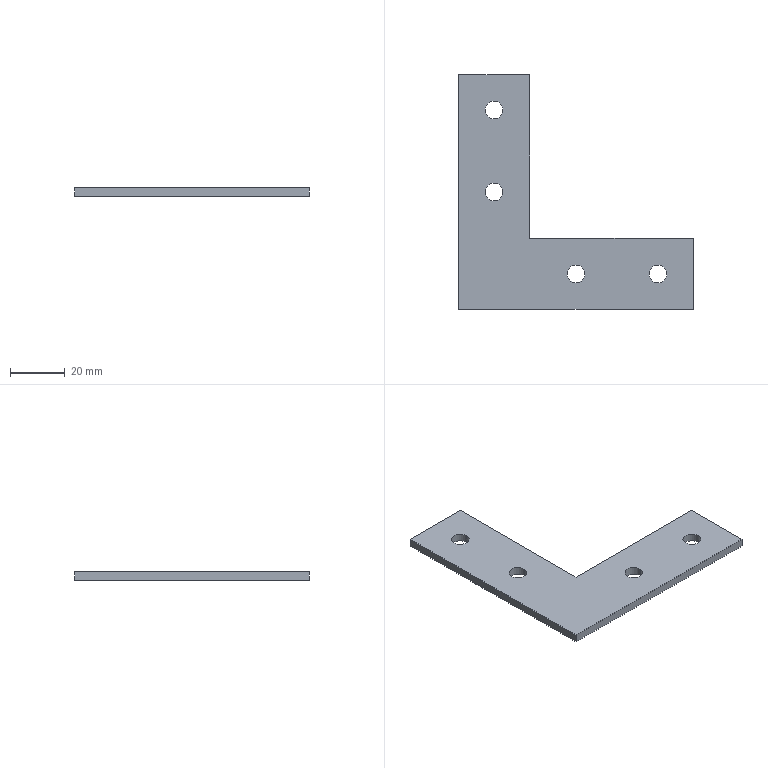Part | STEP file | Outer connecting plate | 1 solid | 16 faces | box 86 x 86 x 3 mm | volume 10990 mm3 | cylinder 8 | plane 8 | commonest cylinder face diameters 6.5 x8
STEP:
#1=CARTESIAN_POINT('',(0.,0.,0.));
#2=DIRECTION('',(0.,0.,1.));
#3=DIRECTION('',(1.,0.,0.));
#4=AXIS2_PLACEMENT_3D('',#1,#2,#3);
#5=CARTESIAN_POINT('',(16.25,73.,0.));
#6=VERTEX_POINT('',#5);
#7=CARTESIAN_POINT('',(16.25,73.,3.));
#8=VERTEX_POINT('',#7);
#9=CARTESIAN_POINT('',(16.25,73.,3.));
#10=DIRECTION('',(0.,0.,1.));
#11=VECTOR('',#10,1.);
#12=LINE('',#9,#11);
#13=CARTESIAN_POINT('',(13.,73.,3.));
#14=DIRECTION('',(0.,0.,1.));
#15=DIRECTION('',(1.,0.,0.));
#16=AXIS2_PLACEMENT_3D('',#13,#14,#15);
#17=CYLINDRICAL_SURFACE('',#16,3.25);
#18=CARTESIAN_POINT('',(6.283,0.));
#19=DIRECTION('',(0.,1.));
#20=VECTOR('',#19,1.);
#21=LINE('',#18,#20);
#22=(GEOMETRIC_REPRESENTATION_CONTEXT(2)PARAMETRIC_REPRESENTATION_CONTEXT()REPRESENTATION_CONTEXT('',''));
#23=DEFINITIONAL_REPRESENTATION('',(#21),#22);
#24=PCURVE('',#17,#23);
#25=CARTESIAN_POINT('',(13.,73.,3.));
#26=DIRECTION('',(0.,0.,1.));
#27=DIRECTION('',(1.,0.,0.));
#28=AXIS2_PLACEMENT_3D('',#25,#26,#27);
#29=CYLINDRICAL_SURFACE('',#28,3.25);
#30=CARTESIAN_POINT('',(0.,0.));
#31=DIRECTION('',(0.,1.));
#32=VECTOR('',#31,1.);
#33=LINE('',#30,#32);
#34=(GEOMETRIC_REPRESENTATION_CONTEXT(2)PARAMETRIC_REPRESENTATION_CONTEXT()REPRESENTATION_CONTEXT('',''));
#35=DEFINITIONAL_REPRESENTATION('',(#33),#34);
#36=PCURVE('',#29,#35);
#37=SURFACE_CURVE('',#12,(#24,#36),.PCURVE_S1.);
#38=EDGE_CURVE('',#6,#8,#37,.T.);
#39=ORIENTED_EDGE('',*,*,#38,.T.);
#40=CARTESIAN_POINT('',(9.75,73.,3.));
#41=VERTEX_POINT('',#40);
#42=CARTESIAN_POINT('',(13.,73.,3.));
#43=DIRECTION('',(0.,0.,1.));
#44=DIRECTION('',(1.,0.,0.));
#45=AXIS2_PLACEMENT_3D('',#42,#43,#44);
#46=CIRCLE('',#45,3.25);
#47=CARTESIAN_POINT('',(0.,0.));
#48=DIRECTION('',(1.,0.));
#49=VECTOR('',#48,1.);
#50=LINE('',#47,#49);
#51=(GEOMETRIC_REPRESENTATION_CONTEXT(2)PARAMETRIC_REPRESENTATION_CONTEXT()REPRESENTATION_CONTEXT('',''));
#52=DEFINITIONAL_REPRESENTATION('',(#50),#51);
#53=PCURVE('',#17,#52);
#54=CARTESIAN_POINT('',(0.,0.,3.));
#55=DIRECTION('',(0.,0.,-1.));
#56=DIRECTION('',(-1.,0.,0.));
#57=AXIS2_PLACEMENT_3D('',#54,#55,#56);
#58=PLANE('',#57);
#59=CARTESIAN_POINT('',(-16.25,73.));
#60=CARTESIAN_POINT('',(-16.25,78.629));
#61=CARTESIAN_POINT('',(-11.375,75.815));
#62=CARTESIAN_POINT('',(-6.5,73.));
#63=CARTESIAN_POINT('',(-11.375,70.185));
#64=CARTESIAN_POINT('',(-16.25,67.371));
#65=CARTESIAN_POINT('',(-16.25,73.));
#66=(BOUNDED_CURVE()B_SPLINE_CURVE(2,(#59,#60,#61,#62,#63,#64,#65),.UNSPECIFIED.,.T.,.F.)B_SPLINE_CURVE_WITH_KNOTS((1,2,2,2,2,1),(-2.094,0.,2.094,4.189,6.283,8.378),.UNSPECIFIED.)CURVE()GEOMETRIC_REPRESENTATION_ITEM()RATIONAL_B_SPLINE_CURVE((1.,0.5,1.,0.5,1.,0.5,1.))REPRESENTATION_ITEM(''));
#67=(GEOMETRIC_REPRESENTATION_CONTEXT(2)PARAMETRIC_REPRESENTATION_CONTEXT()REPRESENTATION_CONTEXT('',''));
#68=DEFINITIONAL_REPRESENTATION('',(#66),#67);
#69=PCURVE('',#58,#68);
#70=SURFACE_CURVE('',#46,(#53,#69),.PCURVE_S1.);
#71=EDGE_CURVE('',#41,#8,#70,.T.);
#72=ORIENTED_EDGE('',*,*,#71,.F.);
#73=CARTESIAN_POINT('',(9.75,73.,0.));
#74=VERTEX_POINT('',#73);
#75=CARTESIAN_POINT('',(9.75,73.,3.));
#76=DIRECTION('',(0.,0.,1.));
#77=VECTOR('',#76,1.);
#78=LINE('',#75,#77);
#79=CARTESIAN_POINT('',(3.142,0.));
#80=DIRECTION('',(0.,1.));
#81=VECTOR('',#80,1.);
#82=LINE('',#79,#81);
#83=(GEOMETRIC_REPRESENTATION_CONTEXT(2)PARAMETRIC_REPRESENTATION_CONTEXT()REPRESENTATION_CONTEXT('',''));
#84=DEFINITIONAL_REPRESENTATION('',(#82),#83);
#85=PCURVE('',#17,#84);
#86=CARTESIAN_POINT('',(3.142,0.));
#87=DIRECTION('',(0.,1.));
#88=VECTOR('',#87,1.);
#89=LINE('',#86,#88);
#90=(GEOMETRIC_REPRESENTATION_CONTEXT(2)PARAMETRIC_REPRESENTATION_CONTEXT()REPRESENTATION_CONTEXT('',''));
#91=DEFINITIONAL_REPRESENTATION('',(#89),#90);
#92=PCURVE('',#29,#91);
#93=SURFACE_CURVE('',#78,(#85,#92),.PCURVE_S1.);
#94=EDGE_CURVE('',#74,#41,#93,.T.);
#95=ORIENTED_EDGE('',*,*,#94,.F.);
#96=CARTESIAN_POINT('',(13.,73.,0.));
#97=DIRECTION('',(0.,0.,-1.));
#98=DIRECTION('',(-1.,0.,0.));
#99=AXIS2_PLACEMENT_3D('',#96,#97,#98);
#100=CIRCLE('',#99,3.25);
#101=CARTESIAN_POINT('',(9.425,-3.));
#102=DIRECTION('',(-1.,0.));
#103=VECTOR('',#102,1.);
#104=LINE('',#101,#103);
#105=(GEOMETRIC_REPRESENTATION_CONTEXT(2)PARAMETRIC_REPRESENTATION_CONTEXT()REPRESENTATION_CONTEXT('',''));
#106=DEFINITIONAL_REPRESENTATION('',(#104),#105);
#107=PCURVE('',#17,#106);
#108=CARTESIAN_POINT('',(0.,0.,0.));
#109=DIRECTION('',(0.,0.,-1.));
#110=DIRECTION('',(-1.,0.,0.));
#111=AXIS2_PLACEMENT_3D('',#108,#109,#110);
#112=PLANE('',#111);
#113=CARTESIAN_POINT('',(-13.,73.));
#114=DIRECTION('',(1.,0.));
#115=AXIS2_PLACEMENT_2D('',#113,#114);
#116=CIRCLE('',#115,3.25);
#117=(GEOMETRIC_REPRESENTATION_CONTEXT(2)PARAMETRIC_REPRESENTATION_CONTEXT()REPRESENTATION_CONTEXT('',''));
#118=DEFINITIONAL_REPRESENTATION('',(#116),#117);
#119=PCURVE('',#112,#118);
#120=SURFACE_CURVE('',#100,(#107,#119),.PCURVE_S1.);
#121=EDGE_CURVE('',#6,#74,#120,.T.);
#122=ORIENTED_EDGE('',*,*,#121,.F.);
#123=EDGE_LOOP('',(#39,#72,#95,#122));
#124=FACE_BOUND('',#123,.F.);
#125=ADVANCED_FACE('',(#124),#17,.F.);
#126=CARTESIAN_POINT('',(16.25,43.,0.));
#127=VERTEX_POINT('',#126);
#128=CARTESIAN_POINT('',(16.25,43.,3.));
#129=VERTEX_POINT('',#128);
#130=CARTESIAN_POINT('',(16.25,43.,3.));
#131=DIRECTION('',(0.,0.,1.));
#132=VECTOR('',#131,1.);
#133=LINE('',#130,#132);
#134=CARTESIAN_POINT('',(13.,43.,3.));
#135=DIRECTION('',(0.,0.,1.));
#136=DIRECTION('',(1.,0.,0.));
#137=AXIS2_PLACEMENT_3D('',#134,#135,#136);
#138=CYLINDRICAL_SURFACE('',#137,3.25);
#139=CARTESIAN_POINT('',(6.283,0.));
#140=DIRECTION('',(0.,1.));
#141=VECTOR('',#140,1.);
#142=LINE('',#139,#141);
#143=(GEOMETRIC_REPRESENTATION_CONTEXT(2)PARAMETRIC_REPRESENTATION_CONTEXT()REPRESENTATION_CONTEXT('',''));
#144=DEFINITIONAL_REPRESENTATION('',(#142),#143);
#145=PCURVE('',#138,#144);
#146=CARTESIAN_POINT('',(13.,43.,3.));
#147=DIRECTION('',(0.,0.,1.));
#148=DIRECTION('',(1.,0.,0.));
#149=AXIS2_PLACEMENT_3D('',#146,#147,#148);
#150=CYLINDRICAL_SURFACE('',#149,3.25);
#151=CARTESIAN_POINT('',(0.,0.));
#152=DIRECTION('',(0.,1.));
#153=VECTOR('',#152,1.);
#154=LINE('',#151,#153);
#155=(GEOMETRIC_REPRESENTATION_CONTEXT(2)PARAMETRIC_REPRESENTATION_CONTEXT()REPRESENTATION_CONTEXT('',''));
#156=DEFINITIONAL_REPRESENTATION('',(#154),#155);
#157=PCURVE('',#150,#156);
#158=SURFACE_CURVE('',#133,(#145,#157),.PCURVE_S1.);
#159=EDGE_CURVE('',#127,#129,#158,.T.);
#160=ORIENTED_EDGE('',*,*,#159,.T.);
#161=CARTESIAN_POINT('',(9.75,43.,3.));
#162=VERTEX_POINT('',#161);
#163=CARTESIAN_POINT('',(13.,43.,3.));
#164=DIRECTION('',(0.,0.,1.));
#165=DIRECTION('',(1.,0.,0.));
#166=AXIS2_PLACEMENT_3D('',#163,#164,#165);
#167=CIRCLE('',#166,3.25);
#168=CARTESIAN_POINT('',(0.,0.));
#169=DIRECTION('',(1.,0.));
#170=VECTOR('',#169,1.);
#171=LINE('',#168,#170);
#172=(GEOMETRIC_REPRESENTATION_CONTEXT(2)PARAMETRIC_REPRESENTATION_CONTEXT()REPRESENTATION_CONTEXT('',''));
#173=DEFINITIONAL_REPRESENTATION('',(#171),#172);
#174=PCURVE('',#138,#173);
#175=CARTESIAN_POINT('',(-16.25,43.));
#176=CARTESIAN_POINT('',(-16.25,48.629));
#177=CARTESIAN_POINT('',(-11.375,45.815));
#178=CARTESIAN_POINT('',(-6.5,43.));
#179=CARTESIAN_POINT('',(-11.375,40.185));
#180=CARTESIAN_POINT('',(-16.25,37.371));
#181=CARTESIAN_POINT('',(-16.25,43.));
#182=(BOUNDED_CURVE()B_SPLINE_CURVE(2,(#175,#176,#177,#178,#179,#180,#181),.UNSPECIFIED.,.T.,.F.)B_SPLINE_CURVE_WITH_KNOTS((1,2,2,2,2,1),(-2.094,0.,2.094,4.189,6.283,8.378),.UNSPECIFIED.)CURVE()GEOMETRIC_REPRESENTATION_ITEM()RATIONAL_B_SPLINE_CURVE((1.,0.5,1.,0.5,1.,0.5,1.))REPRESENTATION_ITEM(''));
#183=(GEOMETRIC_REPRESENTATION_CONTEXT(2)PARAMETRIC_REPRESENTATION_CONTEXT()REPRESENTATION_CONTEXT('',''));
#184=DEFINITIONAL_REPRESENTATION('',(#182),#183);
#185=PCURVE('',#58,#184);
#186=SURFACE_CURVE('',#167,(#174,#185),.PCURVE_S1.);
#187=EDGE_CURVE('',#162,#129,#186,.T.);
#188=ORIENTED_EDGE('',*,*,#187,.F.);
#189=CARTESIAN_POINT('',(9.75,43.,0.));
#190=VERTEX_POINT('',#189);
#191=CARTESIAN_POINT('',(9.75,43.,3.));
#192=DIRECTION('',(0.,0.,1.));
#193=VECTOR('',#192,1.);
#194=LINE('',#191,#193);
#195=CARTESIAN_POINT('',(3.142,0.));
#196=DIRECTION('',(0.,1.));
#197=VECTOR('',#196,1.);
#198=LINE('',#195,#197);
#199=(GEOMETRIC_REPRESENTATION_CONTEXT(2)PARAMETRIC_REPRESENTATION_CONTEXT()REPRESENTATION_CONTEXT('',''));
#200=DEFINITIONAL_REPRESENTATION('',(#198),#199);
#201=PCURVE('',#138,#200);
#202=CARTESIAN_POINT('',(3.142,0.));
#203=DIRECTION('',(0.,1.));
#204=VECTOR('',#203,1.);
#205=LINE('',#202,#204);
#206=(GEOMETRIC_REPRESENTATION_CONTEXT(2)PARAMETRIC_REPRESENTATION_CONTEXT()REPRESENTATION_CONTEXT('',''));
#207=DEFINITIONAL_REPRESENTATION('',(#205),#206);
#208=PCURVE('',#150,#207);
#209=SURFACE_CURVE('',#194,(#201,#208),.PCURVE_S1.);
#210=EDGE_CURVE('',#190,#162,#209,.T.);
#211=ORIENTED_EDGE('',*,*,#210,.F.);
#212=CARTESIAN_POINT('',(13.,43.,0.));
#213=DIRECTION('',(0.,0.,-1.));
#214=DIRECTION('',(-1.,0.,0.));
#215=AXIS2_PLACEMENT_3D('',#212,#213,#214);
#216=CIRCLE('',#215,3.25);
#217=CARTESIAN_POINT('',(9.425,-3.));
#218=DIRECTION('',(-1.,0.));
#219=VECTOR('',#218,1.);
#220=LINE('',#217,#219);
#221=(GEOMETRIC_REPRESENTATION_CONTEXT(2)PARAMETRIC_REPRESENTATION_CONTEXT()REPRESENTATION_CONTEXT('',''));
#222=DEFINITIONAL_REPRESENTATION('',(#220),#221);
#223=PCURVE('',#138,#222);
#224=CARTESIAN_POINT('',(-13.,43.));
#225=DIRECTION('',(1.,0.));
#226=AXIS2_PLACEMENT_2D('',#224,#225);
#227=CIRCLE('',#226,3.25);
#228=(GEOMETRIC_REPRESENTATION_CONTEXT(2)PARAMETRIC_REPRESENTATION_CONTEXT()REPRESENTATION_CONTEXT('',''));
#229=DEFINITIONAL_REPRESENTATION('',(#227),#228);
#230=PCURVE('',#112,#229);
#231=SURFACE_CURVE('',#216,(#223,#230),.PCURVE_S1.);
#232=EDGE_CURVE('',#127,#190,#231,.T.);
#233=ORIENTED_EDGE('',*,*,#232,.F.);
#234=EDGE_LOOP('',(#160,#188,#211,#233));
#235=FACE_BOUND('',#234,.F.);
#236=ADVANCED_FACE('',(#235),#138,.F.);
#237=CARTESIAN_POINT('',(46.25,13.,0.));
#238=VERTEX_POINT('',#237);
#239=CARTESIAN_POINT('',(46.25,13.,3.));
#240=VERTEX_POINT('',#239);
#241=CARTESIAN_POINT('',(46.25,13.,3.));
#242=DIRECTION('',(0.,0.,1.));
#243=VECTOR('',#242,1.);
#244=LINE('',#241,#243);
#245=CARTESIAN_POINT('',(43.,13.,3.));
#246=DIRECTION('',(0.,0.,1.));
#247=DIRECTION('',(1.,0.,0.));
#248=AXIS2_PLACEMENT_3D('',#245,#246,#247);
#249=CYLINDRICAL_SURFACE('',#248,3.25);
#250=CARTESIAN_POINT('',(6.283,0.));
#251=DIRECTION('',(0.,1.));
#252=VECTOR('',#251,1.);
#253=LINE('',#250,#252);
#254=(GEOMETRIC_REPRESENTATION_CONTEXT(2)PARAMETRIC_REPRESENTATION_CONTEXT()REPRESENTATION_CONTEXT('',''));
#255=DEFINITIONAL_REPRESENTATION('',(#253),#254);
#256=PCURVE('',#249,#255);
#257=CARTESIAN_POINT('',(43.,13.,3.));
#258=DIRECTION('',(0.,0.,1.));
#259=DIRECTION('',(1.,0.,0.));
#260=AXIS2_PLACEMENT_3D('',#257,#258,#259);
#261=CYLINDRICAL_SURFACE('',#260,3.25);
#262=CARTESIAN_POINT('',(0.,0.));
#263=DIRECTION('',(0.,1.));
#264=VECTOR('',#263,1.);
#265=LINE('',#262,#264);
#266=(GEOMETRIC_REPRESENTATION_CONTEXT(2)PARAMETRIC_REPRESENTATION_CONTEXT()REPRESENTATION_CONTEXT('',''));
#267=DEFINITIONAL_REPRESENTATION('',(#265),#266);
#268=PCURVE('',#261,#267);
#269=SURFACE_CURVE('',#244,(#256,#268),.PCURVE_S1.);
#270=EDGE_CURVE('',#238,#240,#269,.T.);
#271=ORIENTED_EDGE('',*,*,#270,.T.);
#272=CARTESIAN_POINT('',(39.75,13.,3.));
#273=VERTEX_POINT('',#272);
#274=CARTESIAN_POINT('',(43.,13.,3.));
#275=DIRECTION('',(0.,0.,1.));
#276=DIRECTION('',(1.,0.,0.));
#277=AXIS2_PLACEMENT_3D('',#274,#275,#276);
#278=CIRCLE('',#277,3.25);
#279=CARTESIAN_POINT('',(0.,0.));
#280=DIRECTION('',(1.,0.));
#281=VECTOR('',#280,1.);
#282=LINE('',#279,#281);
#283=(GEOMETRIC_REPRESENTATION_CONTEXT(2)PARAMETRIC_REPRESENTATION_CONTEXT()REPRESENTATION_CONTEXT('',''));
#284=DEFINITIONAL_REPRESENTATION('',(#282),#283);
#285=PCURVE('',#249,#284);
#286=CARTESIAN_POINT('',(-46.25,13.));
#287=CARTESIAN_POINT('',(-46.25,18.629));
#288=CARTESIAN_POINT('',(-41.375,15.815));
#289=CARTESIAN_POINT('',(-36.5,13.));
#290=CARTESIAN_POINT('',(-41.375,10.185));
#291=CARTESIAN_POINT('',(-46.25,7.371));
#292=CARTESIAN_POINT('',(-46.25,13.));
#293=(BOUNDED_CURVE()B_SPLINE_CURVE(2,(#286,#287,#288,#289,#290,#291,#292),.UNSPECIFIED.,.T.,.F.)B_SPLINE_CURVE_WITH_KNOTS((1,2,2,2,2,1),(-2.094,0.,2.094,4.189,6.283,8.378),.UNSPECIFIED.)CURVE()GEOMETRIC_REPRESENTATION_ITEM()RATIONAL_B_SPLINE_CURVE((1.,0.5,1.,0.5,1.,0.5,1.))REPRESENTATION_ITEM(''));
#294=(GEOMETRIC_REPRESENTATION_CONTEXT(2)PARAMETRIC_REPRESENTATION_CONTEXT()REPRESENTATION_CONTEXT('',''));
#295=DEFINITIONAL_REPRESENTATION('',(#293),#294);
#296=PCURVE('',#58,#295);
#297=SURFACE_CURVE('',#278,(#285,#296),.PCURVE_S1.);
#298=EDGE_CURVE('',#273,#240,#297,.T.);
#299=ORIENTED_EDGE('',*,*,#298,.F.);
#300=CARTESIAN_POINT('',(39.75,13.,0.));
#301=VERTEX_POINT('',#300);
#302=CARTESIAN_POINT('',(39.75,13.,3.));
#303=DIRECTION('',(0.,0.,1.));
#304=VECTOR('',#303,1.);
#305=LINE('',#302,#304);
#306=CARTESIAN_POINT('',(3.142,0.));
#307=DIRECTION('',(0.,1.));
#308=VECTOR('',#307,1.);
#309=LINE('',#306,#308);
#310=(GEOMETRIC_REPRESENTATION_CONTEXT(2)PARAMETRIC_REPRESENTATION_CONTEXT()REPRESENTATION_CONTEXT('',''));
#311=DEFINITIONAL_REPRESENTATION('',(#309),#310);
#312=PCURVE('',#249,#311);
#313=CARTESIAN_POINT('',(3.142,0.));
#314=DIRECTION('',(0.,1.));
#315=VECTOR('',#314,1.);
#316=LINE('',#313,#315);
#317=(GEOMETRIC_REPRESENTATION_CONTEXT(2)PARAMETRIC_REPRESENTATION_CONTEXT()REPRESENTATION_CONTEXT('',''));
#318=DEFINITIONAL_REPRESENTATION('',(#316),#317);
#319=PCURVE('',#261,#318);
#320=SURFACE_CURVE('',#305,(#312,#319),.PCURVE_S1.);
#321=EDGE_CURVE('',#301,#273,#320,.T.);
#322=ORIENTED_EDGE('',*,*,#321,.F.);
#323=CARTESIAN_POINT('',(43.,13.,0.));
#324=DIRECTION('',(0.,0.,-1.));
#325=DIRECTION('',(-1.,0.,0.));
#326=AXIS2_PLACEMENT_3D('',#323,#324,#325);
#327=CIRCLE('',#326,3.25);
#328=CARTESIAN_POINT('',(9.425,-3.));
#329=DIRECTION('',(-1.,0.));
#330=VECTOR('',#329,1.);
#331=LINE('',#328,#330);
#332=(GEOMETRIC_REPRESENTATION_CONTEXT(2)PARAMETRIC_REPRESENTATION_CONTEXT()REPRESENTATION_CONTEXT('',''));
#333=DEFINITIONAL_REPRESENTATION('',(#331),#332);
#334=PCURVE('',#249,#333);
#335=CARTESIAN_POINT('',(-43.,13.));
#336=DIRECTION('',(1.,0.));
#337=AXIS2_PLACEMENT_2D('',#335,#336);
#338=CIRCLE('',#337,3.25);
#339=(GEOMETRIC_REPRESENTATION_CONTEXT(2)PARAMETRIC_REPRESENTATION_CONTEXT()REPRESENTATION_CONTEXT('',''));
#340=DEFINITIONAL_REPRESENTATION('',(#338),#339);
#341=PCURVE('',#112,#340);
#342=SURFACE_CURVE('',#327,(#334,#341),.PCURVE_S1.);
#343=EDGE_CURVE('',#238,#301,#342,.T.);
#344=ORIENTED_EDGE('',*,*,#343,.F.);
#345=EDGE_LOOP('',(#271,#299,#322,#344));
#346=FACE_BOUND('',#345,.F.);
#347=ADVANCED_FACE('',(#346),#249,.F.);
#348=CARTESIAN_POINT('',(76.25,13.,0.));
#349=VERTEX_POINT('',#348);
#350=CARTESIAN_POINT('',(76.25,13.,3.));
#351=VERTEX_POINT('',#350);
#352=CARTESIAN_POINT('',(76.25,13.,3.));
#353=DIRECTION('',(0.,0.,1.));
#354=VECTOR('',#353,1.);
#355=LINE('',#352,#354);
#356=CARTESIAN_POINT('',(73.,13.,3.));
#357=DIRECTION('',(0.,0.,1.));
#358=DIRECTION('',(1.,0.,0.));
#359=AXIS2_PLACEMENT_3D('',#356,#357,#358);
#360=CYLINDRICAL_SURFACE('',#359,3.25);
#361=CARTESIAN_POINT('',(6.283,0.));
#362=DIRECTION('',(0.,1.));
#363=VECTOR('',#362,1.);
#364=LINE('',#361,#363);
#365=(GEOMETRIC_REPRESENTATION_CONTEXT(2)PARAMETRIC_REPRESENTATION_CONTEXT()REPRESENTATION_CONTEXT('',''));
#366=DEFINITIONAL_REPRESENTATION('',(#364),#365);
#367=PCURVE('',#360,#366);
#368=CARTESIAN_POINT('',(73.,13.,3.));
#369=DIRECTION('',(0.,0.,1.));
#370=DIRECTION('',(1.,0.,0.));
#371=AXIS2_PLACEMENT_3D('',#368,#369,#370);
#372=CYLINDRICAL_SURFACE('',#371,3.25);
#373=CARTESIAN_POINT('',(0.,0.));
#374=DIRECTION('',(0.,1.));
#375=VECTOR('',#374,1.);
#376=LINE('',#373,#375);
#377=(GEOMETRIC_REPRESENTATION_CONTEXT(2)PARAMETRIC_REPRESENTATION_CONTEXT()REPRESENTATION_CONTEXT('',''));
#378=DEFINITIONAL_REPRESENTATION('',(#376),#377);
#379=PCURVE('',#372,#378);
#380=SURFACE_CURVE('',#355,(#367,#379),.PCURVE_S1.);
#381=EDGE_CURVE('',#349,#351,#380,.T.);
#382=ORIENTED_EDGE('',*,*,#381,.T.);
#383=CARTESIAN_POINT('',(69.75,13.,3.));
#384=VERTEX_POINT('',#383);
#385=CARTESIAN_POINT('',(73.,13.,3.));
#386=DIRECTION('',(0.,0.,1.));
#387=DIRECTION('',(1.,0.,0.));
#388=AXIS2_PLACEMENT_3D('',#385,#386,#387);
#389=CIRCLE('',#388,3.25);
#390=CARTESIAN_POINT('',(0.,0.));
#391=DIRECTION('',(1.,0.));
#392=VECTOR('',#391,1.);
#393=LINE('',#390,#392);
#394=(GEOMETRIC_REPRESENTATION_CONTEXT(2)PARAMETRIC_REPRESENTATION_CONTEXT()REPRESENTATION_CONTEXT('',''));
#395=DEFINITIONAL_REPRESENTATION('',(#393),#394);
#396=PCURVE('',#360,#395);
#397=CARTESIAN_POINT('',(-76.25,13.));
#398=CARTESIAN_POINT('',(-76.25,18.629));
#399=CARTESIAN_POINT('',(-71.375,15.815));
#400=CARTESIAN_POINT('',(-66.5,13.));
#401=CARTESIAN_POINT('',(-71.375,10.185));
#402=CARTESIAN_POINT('',(-76.25,7.371));
#403=CARTESIAN_POINT('',(-76.25,13.));
#404=(BOUNDED_CURVE()B_SPLINE_CURVE(2,(#397,#398,#399,#400,#401,#402,#403),.UNSPECIFIED.,.T.,.F.)B_SPLINE_CURVE_WITH_KNOTS((1,2,2,2,2,1),(-2.094,0.,2.094,4.189,6.283,8.378),.UNSPECIFIED.)CURVE()GEOMETRIC_REPRESENTATION_ITEM()RATIONAL_B_SPLINE_CURVE((1.,0.5,1.,0.5,1.,0.5,1.))REPRESENTATION_ITEM(''));
#405=(GEOMETRIC_REPRESENTATION_CONTEXT(2)PARAMETRIC_REPRESENTATION_CONTEXT()REPRESENTATION_CONTEXT('',''));
#406=DEFINITIONAL_REPRESENTATION('',(#404),#405);
#407=PCURVE('',#58,#406);
#408=SURFACE_CURVE('',#389,(#396,#407),.PCURVE_S1.);
#409=EDGE_CURVE('',#384,#351,#408,.T.);
#410=ORIENTED_EDGE('',*,*,#409,.F.);
#411=CARTESIAN_POINT('',(69.75,13.,0.));
#412=VERTEX_POINT('',#411);
#413=CARTESIAN_POINT('',(69.75,13.,3.));
#414=DIRECTION('',(0.,0.,1.));
#415=VECTOR('',#414,1.);
#416=LINE('',#413,#415);
#417=CARTESIAN_POINT('',(3.142,0.));
#418=DIRECTION('',(0.,1.));
#419=VECTOR('',#418,1.);
#420=LINE('',#417,#419);
#421=(GEOMETRIC_REPRESENTATION_CONTEXT(2)PARAMETRIC_REPRESENTATION_CONTEXT()REPRESENTATION_CONTEXT('',''));
#422=DEFINITIONAL_REPRESENTATION('',(#420),#421);
#423=PCURVE('',#360,#422);
#424=CARTESIAN_POINT('',(3.142,0.));
#425=DIRECTION('',(0.,1.));
#426=VECTOR('',#425,1.);
#427=LINE('',#424,#426);
#428=(GEOMETRIC_REPRESENTATION_CONTEXT(2)PARAMETRIC_REPRESENTATION_CONTEXT()REPRESENTATION_CONTEXT('',''));
#429=DEFINITIONAL_REPRESENTATION('',(#427),#428);
#430=PCURVE('',#372,#429);
#431=SURFACE_CURVE('',#416,(#423,#430),.PCURVE_S1.);
#432=EDGE_CURVE('',#412,#384,#431,.T.);
#433=ORIENTED_EDGE('',*,*,#432,.F.);
#434=CARTESIAN_POINT('',(73.,13.,0.));
#435=DIRECTION('',(0.,0.,-1.));
#436=DIRECTION('',(-1.,0.,0.));
#437=AXIS2_PLACEMENT_3D('',#434,#435,#436);
#438=CIRCLE('',#437,3.25);
#439=CARTESIAN_POINT('',(9.425,-3.));
#440=DIRECTION('',(-1.,0.));
#441=VECTOR('',#440,1.);
#442=LINE('',#439,#441);
#443=(GEOMETRIC_REPRESENTATION_CONTEXT(2)PARAMETRIC_REPRESENTATION_CONTEXT()REPRESENTATION_CONTEXT('',''));
#444=DEFINITIONAL_REPRESENTATION('',(#442),#443);
#445=PCURVE('',#360,#444);
#446=CARTESIAN_POINT('',(-73.,13.));
#447=DIRECTION('',(1.,0.));
#448=AXIS2_PLACEMENT_2D('',#446,#447);
#449=CIRCLE('',#448,3.25);
#450=(GEOMETRIC_REPRESENTATION_CONTEXT(2)PARAMETRIC_REPRESENTATION_CONTEXT()REPRESENTATION_CONTEXT('',''));
#451=DEFINITIONAL_REPRESENTATION('',(#449),#450);
#452=PCURVE('',#112,#451);
#453=SURFACE_CURVE('',#438,(#445,#452),.PCURVE_S1.);
#454=EDGE_CURVE('',#349,#412,#453,.T.);
#455=ORIENTED_EDGE('',*,*,#454,.F.);
#456=EDGE_LOOP('',(#382,#410,#433,#455));
#457=FACE_BOUND('',#456,.F.);
#458=ADVANCED_FACE('',(#457),#360,.F.);
#459=CARTESIAN_POINT('',(0.,0.,0.));
#460=VERTEX_POINT('',#459);
#461=CARTESIAN_POINT('',(86.,0.,0.));
#462=VERTEX_POINT('',#461);
#463=CARTESIAN_POINT('',(86.,0.,0.));
#464=DIRECTION('',(1.,0.,0.));
#465=VECTOR('',#464,1.);
#466=LINE('',#463,#465);
#467=CARTESIAN_POINT('',(86.,0.,3.));
#468=DIRECTION('',(0.,1.,0.));
#469=DIRECTION('',(-1.,0.,0.));
#470=AXIS2_PLACEMENT_3D('',#467,#468,#469);
#471=PLANE('',#470);
#472=CARTESIAN_POINT('',(0.,-3.));
#473=DIRECTION('',(-1.,0.));
#474=VECTOR('',#473,1.);
#475=LINE('',#472,#474);
#476=(GEOMETRIC_REPRESENTATION_CONTEXT(2)PARAMETRIC_REPRESENTATION_CONTEXT()REPRESENTATION_CONTEXT('',''));
#477=DEFINITIONAL_REPRESENTATION('',(#475),#476);
#478=PCURVE('',#471,#477);
#479=CARTESIAN_POINT('',(-86.,0.));
#480=DIRECTION('',(-1.,0.));
#481=VECTOR('',#480,1.);
#482=LINE('',#479,#481);
#483=(GEOMETRIC_REPRESENTATION_CONTEXT(2)PARAMETRIC_REPRESENTATION_CONTEXT()REPRESENTATION_CONTEXT('',''));
#484=DEFINITIONAL_REPRESENTATION('',(#482),#483);
#485=PCURVE('',#112,#484);
#486=SURFACE_CURVE('',#466,(#478,#485),.PCURVE_S1.);
#487=EDGE_CURVE('',#460,#462,#486,.T.);
#488=ORIENTED_EDGE('',*,*,#487,.T.);
#489=CARTESIAN_POINT('',(86.,0.,3.));
#490=VERTEX_POINT('',#489);
#491=CARTESIAN_POINT('',(86.,0.,3.));
#492=DIRECTION('',(0.,0.,-1.));
#493=VECTOR('',#492,1.);
#494=LINE('',#491,#493);
#495=CARTESIAN_POINT('',(0.,0.));
#496=DIRECTION('',(0.,-1.));
#497=VECTOR('',#496,1.);
#498=LINE('',#495,#497);
#499=(GEOMETRIC_REPRESENTATION_CONTEXT(2)PARAMETRIC_REPRESENTATION_CONTEXT()REPRESENTATION_CONTEXT('',''));
#500=DEFINITIONAL_REPRESENTATION('',(#498),#499);
#501=PCURVE('',#471,#500);
#502=CARTESIAN_POINT('',(86.,26.,3.));
#503=DIRECTION('',(-1.,0.,0.));
#504=DIRECTION('',(0.,0.,1.));
#505=AXIS2_PLACEMENT_3D('',#502,#503,#504);
#506=PLANE('',#505);
#507=CARTESIAN_POINT('',(0.,-26.));
#508=DIRECTION('',(-1.,0.));
#509=VECTOR('',#508,1.);
#510=LINE('',#507,#509);
#511=(GEOMETRIC_REPRESENTATION_CONTEXT(2)PARAMETRIC_REPRESENTATION_CONTEXT()REPRESENTATION_CONTEXT('',''));
#512=DEFINITIONAL_REPRESENTATION('',(#510),#511);
#513=PCURVE('',#506,#512);
#514=SURFACE_CURVE('',#494,(#501,#513),.PCURVE_S1.);
#515=EDGE_CURVE('',#490,#462,#514,.T.);
#516=ORIENTED_EDGE('',*,*,#515,.F.);
#517=CARTESIAN_POINT('',(0.,0.,3.));
#518=VERTEX_POINT('',#517);
#519=CARTESIAN_POINT('',(86.,0.,3.));
#520=DIRECTION('',(1.,0.,0.));
#521=VECTOR('',#520,1.);
#522=LINE('',#519,#521);
#523=CARTESIAN_POINT('',(0.,0.));
#524=DIRECTION('',(-1.,0.));
#525=VECTOR('',#524,1.);
#526=LINE('',#523,#525);
#527=(GEOMETRIC_REPRESENTATION_CONTEXT(2)PARAMETRIC_REPRESENTATION_CONTEXT()REPRESENTATION_CONTEXT('',''));
#528=DEFINITIONAL_REPRESENTATION('',(#526),#527);
#529=PCURVE('',#471,#528);
#530=CARTESIAN_POINT('',(-86.,0.));
#531=DIRECTION('',(-1.,0.));
#532=VECTOR('',#531,1.);
#533=LINE('',#530,#532);
#534=(GEOMETRIC_REPRESENTATION_CONTEXT(2)PARAMETRIC_REPRESENTATION_CONTEXT()REPRESENTATION_CONTEXT('',''));
#535=DEFINITIONAL_REPRESENTATION('',(#533),#534);
#536=PCURVE('',#58,#535);
#537=SURFACE_CURVE('',#522,(#529,#536),.PCURVE_S1.);
#538=EDGE_CURVE('',#518,#490,#537,.T.);
#539=ORIENTED_EDGE('',*,*,#538,.F.);
#540=CARTESIAN_POINT('',(0.,0.,3.));
#541=DIRECTION('',(0.,0.,-1.));
#542=VECTOR('',#541,1.);
#543=LINE('',#540,#542);
#544=CARTESIAN_POINT('',(86.,0.));
#545=DIRECTION('',(0.,-1.));
#546=VECTOR('',#545,1.);
#547=LINE('',#544,#546);
#548=(GEOMETRIC_REPRESENTATION_CONTEXT(2)PARAMETRIC_REPRESENTATION_CONTEXT()REPRESENTATION_CONTEXT('',''));
#549=DEFINITIONAL_REPRESENTATION('',(#547),#548);
#550=PCURVE('',#471,#549);
#551=CARTESIAN_POINT('',(0.,0.,3.));
#552=DIRECTION('',(1.,0.,0.));
#553=DIRECTION('',(0.,0.,-1.));
#554=AXIS2_PLACEMENT_3D('',#551,#552,#553);
#555=PLANE('',#554);
#556=CARTESIAN_POINT('',(0.,0.));
#557=DIRECTION('',(1.,0.));
#558=VECTOR('',#557,1.);
#559=LINE('',#556,#558);
#560=(GEOMETRIC_REPRESENTATION_CONTEXT(2)PARAMETRIC_REPRESENTATION_CONTEXT()REPRESENTATION_CONTEXT('',''));
#561=DEFINITIONAL_REPRESENTATION('',(#559),#560);
#562=PCURVE('',#555,#561);
#563=SURFACE_CURVE('',#543,(#550,#562),.PCURVE_S1.);
#564=EDGE_CURVE('',#518,#460,#563,.T.);
#565=ORIENTED_EDGE('',*,*,#564,.T.);
#566=EDGE_LOOP('',(#488,#516,#539,#565));
#567=FACE_BOUND('',#566,.T.);
#568=ADVANCED_FACE('',(#567),#471,.F.);
#569=CARTESIAN_POINT('',(86.,26.,0.));
#570=VERTEX_POINT('',#569);
#571=CARTESIAN_POINT('',(86.,26.,0.));
#572=DIRECTION('',(0.,1.,0.));
#573=VECTOR('',#572,1.);
#574=LINE('',#571,#573);
#575=CARTESIAN_POINT('',(-3.,0.));
#576=DIRECTION('',(0.,1.));
#577=VECTOR('',#576,1.);
#578=LINE('',#575,#577);
#579=(GEOMETRIC_REPRESENTATION_CONTEXT(2)PARAMETRIC_REPRESENTATION_CONTEXT()REPRESENTATION_CONTEXT('',''));
#580=DEFINITIONAL_REPRESENTATION('',(#578),#579);
#581=PCURVE('',#506,#580);
#582=CARTESIAN_POINT('',(-86.,26.));
#583=DIRECTION('',(0.,1.));
#584=VECTOR('',#583,1.);
#585=LINE('',#582,#584);
#586=(GEOMETRIC_REPRESENTATION_CONTEXT(2)PARAMETRIC_REPRESENTATION_CONTEXT()REPRESENTATION_CONTEXT('',''));
#587=DEFINITIONAL_REPRESENTATION('',(#585),#586);
#588=PCURVE('',#112,#587);
#589=SURFACE_CURVE('',#574,(#581,#588),.PCURVE_S1.);
#590=EDGE_CURVE('',#462,#570,#589,.T.);
#591=ORIENTED_EDGE('',*,*,#590,.T.);
#592=CARTESIAN_POINT('',(86.,26.,3.));
#593=VERTEX_POINT('',#592);
#594=CARTESIAN_POINT('',(86.,26.,3.));
#595=DIRECTION('',(0.,0.,-1.));
#596=VECTOR('',#595,1.);
#597=LINE('',#594,#596);
#598=CARTESIAN_POINT('',(0.,0.));
#599=DIRECTION('',(-1.,0.));
#600=VECTOR('',#599,1.);
#601=LINE('',#598,#600);
#602=(GEOMETRIC_REPRESENTATION_CONTEXT(2)PARAMETRIC_REPRESENTATION_CONTEXT()REPRESENTATION_CONTEXT('',''));
#603=DEFINITIONAL_REPRESENTATION('',(#601),#602);
#604=PCURVE('',#506,#603);
#605=CARTESIAN_POINT('',(26.,26.,3.));
#606=DIRECTION('',(0.,-1.,0.));
#607=DIRECTION('',(1.,0.,0.));
#608=AXIS2_PLACEMENT_3D('',#605,#606,#607);
#609=PLANE('',#608);
#610=CARTESIAN_POINT('',(60.,0.));
#611=DIRECTION('',(0.,-1.));
#612=VECTOR('',#611,1.);
#613=LINE('',#610,#612);
#614=(GEOMETRIC_REPRESENTATION_CONTEXT(2)PARAMETRIC_REPRESENTATION_CONTEXT()REPRESENTATION_CONTEXT('',''));
#615=DEFINITIONAL_REPRESENTATION('',(#613),#614);
#616=PCURVE('',#609,#615);
#617=SURFACE_CURVE('',#597,(#604,#616),.PCURVE_S1.);
#618=EDGE_CURVE('',#593,#570,#617,.T.);
#619=ORIENTED_EDGE('',*,*,#618,.F.);
#620=CARTESIAN_POINT('',(86.,26.,3.));
#621=DIRECTION('',(0.,1.,0.));
#622=VECTOR('',#621,1.);
#623=LINE('',#620,#622);
#624=CARTESIAN_POINT('',(0.,0.));
#625=DIRECTION('',(0.,1.));
#626=VECTOR('',#625,1.);
#627=LINE('',#624,#626);
#628=(GEOMETRIC_REPRESENTATION_CONTEXT(2)PARAMETRIC_REPRESENTATION_CONTEXT()REPRESENTATION_CONTEXT('',''));
#629=DEFINITIONAL_REPRESENTATION('',(#627),#628);
#630=PCURVE('',#506,#629);
#631=CARTESIAN_POINT('',(-86.,26.));
#632=DIRECTION('',(0.,1.));
#633=VECTOR('',#632,1.);
#634=LINE('',#631,#633);
#635=(GEOMETRIC_REPRESENTATION_CONTEXT(2)PARAMETRIC_REPRESENTATION_CONTEXT()REPRESENTATION_CONTEXT('',''));
#636=DEFINITIONAL_REPRESENTATION('',(#634),#635);
#637=PCURVE('',#58,#636);
#638=SURFACE_CURVE('',#623,(#630,#637),.PCURVE_S1.);
#639=EDGE_CURVE('',#490,#593,#638,.T.);
#640=ORIENTED_EDGE('',*,*,#639,.F.);
#641=ORIENTED_EDGE('',*,*,#515,.T.);
#642=EDGE_LOOP('',(#591,#619,#640,#641));
#643=FACE_BOUND('',#642,.T.);
#644=ADVANCED_FACE('',(#643),#506,.F.);
#645=CARTESIAN_POINT('',(26.,26.,0.));
#646=VERTEX_POINT('',#645);
#647=CARTESIAN_POINT('',(26.,26.,0.));
#648=DIRECTION('',(-1.,0.,0.));
#649=VECTOR('',#648,1.);
#650=LINE('',#647,#649);
#651=CARTESIAN_POINT('',(0.,-3.));
#652=DIRECTION('',(-1.,0.));
#653=VECTOR('',#652,1.);
#654=LINE('',#651,#653);
#655=(GEOMETRIC_REPRESENTATION_CONTEXT(2)PARAMETRIC_REPRESENTATION_CONTEXT()REPRESENTATION_CONTEXT('',''));
#656=DEFINITIONAL_REPRESENTATION('',(#654),#655);
#657=PCURVE('',#609,#656);
#658=CARTESIAN_POINT('',(-26.,26.));
#659=DIRECTION('',(1.,0.));
#660=VECTOR('',#659,1.);
#661=LINE('',#658,#660);
#662=(GEOMETRIC_REPRESENTATION_CONTEXT(2)PARAMETRIC_REPRESENTATION_CONTEXT()REPRESENTATION_CONTEXT('',''));
#663=DEFINITIONAL_REPRESENTATION('',(#661),#662);
#664=PCURVE('',#112,#663);
#665=SURFACE_CURVE('',#650,(#657,#664),.PCURVE_S1.);
#666=EDGE_CURVE('',#570,#646,#665,.T.);
#667=ORIENTED_EDGE('',*,*,#666,.T.);
#668=CARTESIAN_POINT('',(26.,26.,3.));
#669=VERTEX_POINT('',#668);
#670=CARTESIAN_POINT('',(26.,26.,3.));
#671=DIRECTION('',(0.,0.,-1.));
#672=VECTOR('',#671,1.);
#673=LINE('',#670,#672);
#674=CARTESIAN_POINT('',(0.,0.));
#675=DIRECTION('',(0.,-1.));
#676=VECTOR('',#675,1.);
#677=LINE('',#674,#676);
#678=(GEOMETRIC_REPRESENTATION_CONTEXT(2)PARAMETRIC_REPRESENTATION_CONTEXT()REPRESENTATION_CONTEXT('',''));
#679=DEFINITIONAL_REPRESENTATION('',(#677),#678);
#680=PCURVE('',#609,#679);
#681=CARTESIAN_POINT('',(26.,86.,3.));
#682=DIRECTION('',(-1.,0.,0.));
#683=DIRECTION('',(0.,-1.,0.));
#684=AXIS2_PLACEMENT_3D('',#681,#682,#683);
#685=PLANE('',#684);
#686=CARTESIAN_POINT('',(60.,0.));
#687=DIRECTION('',(0.,-1.));
#688=VECTOR('',#687,1.);
#689=LINE('',#686,#688);
#690=(GEOMETRIC_REPRESENTATION_CONTEXT(2)PARAMETRIC_REPRESENTATION_CONTEXT()REPRESENTATION_CONTEXT('',''));
#691=DEFINITIONAL_REPRESENTATION('',(#689),#690);
#692=PCURVE('',#685,#691);
#693=SURFACE_CURVE('',#673,(#680,#692),.PCURVE_S1.);
#694=EDGE_CURVE('',#669,#646,#693,.T.);
#695=ORIENTED_EDGE('',*,*,#694,.F.);
#696=CARTESIAN_POINT('',(26.,26.,3.));
#697=DIRECTION('',(-1.,0.,0.));
#698=VECTOR('',#697,1.);
#699=LINE('',#696,#698);
#700=CARTESIAN_POINT('',(0.,0.));
#701=DIRECTION('',(-1.,0.));
#702=VECTOR('',#701,1.);
#703=LINE('',#700,#702);
#704=(GEOMETRIC_REPRESENTATION_CONTEXT(2)PARAMETRIC_REPRESENTATION_CONTEXT()REPRESENTATION_CONTEXT('',''));
#705=DEFINITIONAL_REPRESENTATION('',(#703),#704);
#706=PCURVE('',#609,#705);
#707=CARTESIAN_POINT('',(-26.,26.));
#708=DIRECTION('',(1.,0.));
#709=VECTOR('',#708,1.);
#710=LINE('',#707,#709);
#711=(GEOMETRIC_REPRESENTATION_CONTEXT(2)PARAMETRIC_REPRESENTATION_CONTEXT()REPRESENTATION_CONTEXT('',''));
#712=DEFINITIONAL_REPRESENTATION('',(#710),#711);
#713=PCURVE('',#58,#712);
#714=SURFACE_CURVE('',#699,(#706,#713),.PCURVE_S1.);
#715=EDGE_CURVE('',#593,#669,#714,.T.);
#716=ORIENTED_EDGE('',*,*,#715,.F.);
#717=ORIENTED_EDGE('',*,*,#618,.T.);
#718=EDGE_LOOP('',(#667,#695,#716,#717));
#719=FACE_BOUND('',#718,.T.);
#720=ADVANCED_FACE('',(#719),#609,.F.);
#721=CARTESIAN_POINT('',(26.,86.,0.));
#722=VERTEX_POINT('',#721);
#723=CARTESIAN_POINT('',(26.,86.,0.));
#724=DIRECTION('',(0.,1.,0.));
#725=VECTOR('',#724,1.);
#726=LINE('',#723,#725);
#727=CARTESIAN_POINT('',(0.,-3.));
#728=DIRECTION('',(-1.,0.));
#729=VECTOR('',#728,1.);
#730=LINE('',#727,#729);
#731=(GEOMETRIC_REPRESENTATION_CONTEXT(2)PARAMETRIC_REPRESENTATION_CONTEXT()REPRESENTATION_CONTEXT('',''));
#732=DEFINITIONAL_REPRESENTATION('',(#730),#731);
#733=PCURVE('',#685,#732);
#734=CARTESIAN_POINT('',(-26.,86.));
#735=DIRECTION('',(0.,1.));
#736=VECTOR('',#735,1.);
#737=LINE('',#734,#736);
#738=(GEOMETRIC_REPRESENTATION_CONTEXT(2)PARAMETRIC_REPRESENTATION_CONTEXT()REPRESENTATION_CONTEXT('',''));
#739=DEFINITIONAL_REPRESENTATION('',(#737),#738);
#740=PCURVE('',#112,#739);
#741=SURFACE_CURVE('',#726,(#733,#740),.PCURVE_S1.);
#742=EDGE_CURVE('',#646,#722,#741,.T.);
#743=ORIENTED_EDGE('',*,*,#742,.T.);
#744=CARTESIAN_POINT('',(26.,86.,3.));
#745=VERTEX_POINT('',#744);
#746=CARTESIAN_POINT('',(26.,86.,3.));
#747=DIRECTION('',(0.,0.,-1.));
#748=VECTOR('',#747,1.);
#749=LINE('',#746,#748);
#750=CARTESIAN_POINT('',(0.,0.));
#751=DIRECTION('',(0.,-1.));
#752=VECTOR('',#751,1.);
#753=LINE('',#750,#752);
#754=(GEOMETRIC_REPRESENTATION_CONTEXT(2)PARAMETRIC_REPRESENTATION_CONTEXT()REPRESENTATION_CONTEXT('',''));
#755=DEFINITIONAL_REPRESENTATION('',(#753),#754);
#756=PCURVE('',#685,#755);
#757=CARTESIAN_POINT('',(0.,86.,3.));
#758=DIRECTION('',(0.,-1.,0.));
#759=DIRECTION('',(0.,0.,-1.));
#760=AXIS2_PLACEMENT_3D('',#757,#758,#759);
#761=PLANE('',#760);
#762=CARTESIAN_POINT('',(0.,26.));
#763=DIRECTION('',(1.,0.));
#764=VECTOR('',#763,1.);
#765=LINE('',#762,#764);
#766=(GEOMETRIC_REPRESENTATION_CONTEXT(2)PARAMETRIC_REPRESENTATION_CONTEXT()REPRESENTATION_CONTEXT('',''));
#767=DEFINITIONAL_REPRESENTATION('',(#765),#766);
#768=PCURVE('',#761,#767);
#769=SURFACE_CURVE('',#749,(#756,#768),.PCURVE_S1.);
#770=EDGE_CURVE('',#745,#722,#769,.T.);
#771=ORIENTED_EDGE('',*,*,#770,.F.);
#772=CARTESIAN_POINT('',(26.,86.,3.));
#773=DIRECTION('',(0.,1.,0.));
#774=VECTOR('',#773,1.);
#775=LINE('',#772,#774);
#776=CARTESIAN_POINT('',(0.,0.));
#777=DIRECTION('',(-1.,0.));
#778=VECTOR('',#777,1.);
#779=LINE('',#776,#778);
#780=(GEOMETRIC_REPRESENTATION_CONTEXT(2)PARAMETRIC_REPRESENTATION_CONTEXT()REPRESENTATION_CONTEXT('',''));
#781=DEFINITIONAL_REPRESENTATION('',(#779),#780);
#782=PCURVE('',#685,#781);
#783=CARTESIAN_POINT('',(-26.,86.));
#784=DIRECTION('',(0.,1.));
#785=VECTOR('',#784,1.);
#786=LINE('',#783,#785);
#787=(GEOMETRIC_REPRESENTATION_CONTEXT(2)PARAMETRIC_REPRESENTATION_CONTEXT()REPRESENTATION_CONTEXT('',''));
#788=DEFINITIONAL_REPRESENTATION('',(#786),#787);
#789=PCURVE('',#58,#788);
#790=SURFACE_CURVE('',#775,(#782,#789),.PCURVE_S1.);
#791=EDGE_CURVE('',#669,#745,#790,.T.);
#792=ORIENTED_EDGE('',*,*,#791,.F.);
#793=ORIENTED_EDGE('',*,*,#694,.T.);
#794=EDGE_LOOP('',(#743,#771,#792,#793));
#795=FACE_BOUND('',#794,.T.);
#796=ADVANCED_FACE('',(#795),#685,.F.);
#797=CARTESIAN_POINT('',(0.,86.,0.));
#798=VERTEX_POINT('',#797);
#799=CARTESIAN_POINT('',(0.,86.,0.));
#800=DIRECTION('',(-1.,0.,0.));
#801=VECTOR('',#800,1.);
#802=LINE('',#799,#801);
#803=CARTESIAN_POINT('',(3.,0.));
#804=DIRECTION('',(0.,-1.));
#805=VECTOR('',#804,1.);
#806=LINE('',#803,#805);
#807=(GEOMETRIC_REPRESENTATION_CONTEXT(2)PARAMETRIC_REPRESENTATION_CONTEXT()REPRESENTATION_CONTEXT('',''));
#808=DEFINITIONAL_REPRESENTATION('',(#806),#807);
#809=PCURVE('',#761,#808);
#810=CARTESIAN_POINT('',(0.,86.));
#811=DIRECTION('',(1.,0.));
#812=VECTOR('',#811,1.);
#813=LINE('',#810,#812);
#814=(GEOMETRIC_REPRESENTATION_CONTEXT(2)PARAMETRIC_REPRESENTATION_CONTEXT()REPRESENTATION_CONTEXT('',''));
#815=DEFINITIONAL_REPRESENTATION('',(#813),#814);
#816=PCURVE('',#112,#815);
#817=SURFACE_CURVE('',#802,(#809,#816),.PCURVE_S1.);
#818=EDGE_CURVE('',#722,#798,#817,.T.);
#819=ORIENTED_EDGE('',*,*,#818,.T.);
#820=CARTESIAN_POINT('',(0.,86.,3.));
#821=VERTEX_POINT('',#820);
#822=CARTESIAN_POINT('',(0.,86.,3.));
#823=DIRECTION('',(0.,0.,-1.));
#824=VECTOR('',#823,1.);
#825=LINE('',#822,#824);
#826=CARTESIAN_POINT('',(0.,0.));
#827=DIRECTION('',(1.,0.));
#828=VECTOR('',#827,1.);
#829=LINE('',#826,#828);
#830=(GEOMETRIC_REPRESENTATION_CONTEXT(2)PARAMETRIC_REPRESENTATION_CONTEXT()REPRESENTATION_CONTEXT('',''));
#831=DEFINITIONAL_REPRESENTATION('',(#829),#830);
#832=PCURVE('',#761,#831);
#833=CARTESIAN_POINT('',(0.,86.));
#834=DIRECTION('',(1.,0.));
#835=VECTOR('',#834,1.);
#836=LINE('',#833,#835);
#837=(GEOMETRIC_REPRESENTATION_CONTEXT(2)PARAMETRIC_REPRESENTATION_CONTEXT()REPRESENTATION_CONTEXT('',''));
#838=DEFINITIONAL_REPRESENTATION('',(#836),#837);
#839=PCURVE('',#555,#838);
#840=SURFACE_CURVE('',#825,(#832,#839),.PCURVE_S1.);
#841=EDGE_CURVE('',#821,#798,#840,.T.);
#842=ORIENTED_EDGE('',*,*,#841,.F.);
#843=CARTESIAN_POINT('',(0.,86.,3.));
#844=DIRECTION('',(-1.,0.,0.));
#845=VECTOR('',#844,1.);
#846=LINE('',#843,#845);
#847=CARTESIAN_POINT('',(0.,0.));
#848=DIRECTION('',(0.,-1.));
#849=VECTOR('',#848,1.);
#850=LINE('',#847,#849);
#851=(GEOMETRIC_REPRESENTATION_CONTEXT(2)PARAMETRIC_REPRESENTATION_CONTEXT()REPRESENTATION_CONTEXT('',''));
#852=DEFINITIONAL_REPRESENTATION('',(#850),#851);
#853=PCURVE('',#761,#852);
#854=CARTESIAN_POINT('',(0.,86.));
#855=DIRECTION('',(1.,0.));
#856=VECTOR('',#855,1.);
#857=LINE('',#854,#856);
#858=(GEOMETRIC_REPRESENTATION_CONTEXT(2)PARAMETRIC_REPRESENTATION_CONTEXT()REPRESENTATION_CONTEXT('',''));
#859=DEFINITIONAL_REPRESENTATION('',(#857),#858);
#860=PCURVE('',#58,#859);
#861=SURFACE_CURVE('',#846,(#853,#860),.PCURVE_S1.);
#862=EDGE_CURVE('',#745,#821,#861,.T.);
#863=ORIENTED_EDGE('',*,*,#862,.F.);
#864=ORIENTED_EDGE('',*,*,#770,.T.);
#865=EDGE_LOOP('',(#819,#842,#863,#864));
#866=FACE_BOUND('',#865,.T.);
#867=ADVANCED_FACE('',(#866),#761,.F.);
#868=CARTESIAN_POINT('',(0.,0.,0.));
#869=DIRECTION('',(0.,-1.,0.));
#870=VECTOR('',#869,1.);
#871=LINE('',#868,#870);
#872=CARTESIAN_POINT('',(3.,0.));
#873=DIRECTION('',(0.,-1.));
#874=VECTOR('',#873,1.);
#875=LINE('',#872,#874);
#876=(GEOMETRIC_REPRESENTATION_CONTEXT(2)PARAMETRIC_REPRESENTATION_CONTEXT()REPRESENTATION_CONTEXT('',''));
#877=DEFINITIONAL_REPRESENTATION('',(#875),#876);
#878=PCURVE('',#555,#877);
#879=CARTESIAN_POINT('',(0.,0.));
#880=DIRECTION('',(0.,-1.));
#881=VECTOR('',#880,1.);
#882=LINE('',#879,#881);
#883=(GEOMETRIC_REPRESENTATION_CONTEXT(2)PARAMETRIC_REPRESENTATION_CONTEXT()REPRESENTATION_CONTEXT('',''));
#884=DEFINITIONAL_REPRESENTATION('',(#882),#883);
#885=PCURVE('',#112,#884);
#886=SURFACE_CURVE('',#871,(#878,#885),.PCURVE_S1.);
#887=EDGE_CURVE('',#798,#460,#886,.T.);
#888=ORIENTED_EDGE('',*,*,#887,.T.);
#889=ORIENTED_EDGE('',*,*,#564,.F.);
#890=CARTESIAN_POINT('',(0.,0.,3.));
#891=DIRECTION('',(0.,-1.,0.));
#892=VECTOR('',#891,1.);
#893=LINE('',#890,#892);
#894=CARTESIAN_POINT('',(0.,0.));
#895=DIRECTION('',(0.,-1.));
#896=VECTOR('',#895,1.);
#897=LINE('',#894,#896);
#898=(GEOMETRIC_REPRESENTATION_CONTEXT(2)PARAMETRIC_REPRESENTATION_CONTEXT()REPRESENTATION_CONTEXT('',''));
#899=DEFINITIONAL_REPRESENTATION('',(#897),#898);
#900=PCURVE('',#555,#899);
#901=CARTESIAN_POINT('',(0.,0.));
#902=DIRECTION('',(0.,-1.));
#903=VECTOR('',#902,1.);
#904=LINE('',#901,#903);
#905=(GEOMETRIC_REPRESENTATION_CONTEXT(2)PARAMETRIC_REPRESENTATION_CONTEXT()REPRESENTATION_CONTEXT('',''));
#906=DEFINITIONAL_REPRESENTATION('',(#904),#905);
#907=PCURVE('',#58,#906);
#908=SURFACE_CURVE('',#893,(#900,#907),.PCURVE_S1.);
#909=EDGE_CURVE('',#821,#518,#908,.T.);
#910=ORIENTED_EDGE('',*,*,#909,.F.);
#911=ORIENTED_EDGE('',*,*,#841,.T.);
#912=EDGE_LOOP('',(#888,#889,#910,#911));
#913=FACE_BOUND('',#912,.T.);
#914=ADVANCED_FACE('',(#913),#555,.F.);
#915=CARTESIAN_POINT('',(13.,73.,3.));
#916=DIRECTION('',(0.,0.,1.));
#917=DIRECTION('',(1.,0.,0.));
#918=AXIS2_PLACEMENT_3D('',#915,#916,#917);
#919=CIRCLE('',#918,3.25);
#920=CARTESIAN_POINT('',(-16.25,73.));
#921=CARTESIAN_POINT('',(-16.25,78.629));
#922=CARTESIAN_POINT('',(-11.375,75.815));
#923=CARTESIAN_POINT('',(-6.5,73.));
#924=CARTESIAN_POINT('',(-11.375,70.185));
#925=CARTESIAN_POINT('',(-16.25,67.371));
#926=CARTESIAN_POINT('',(-16.25,73.));
#927=(BOUNDED_CURVE()B_SPLINE_CURVE(2,(#920,#921,#922,#923,#924,#925,#926),.UNSPECIFIED.,.T.,.F.)B_SPLINE_CURVE_WITH_KNOTS((1,2,2,2,2,1),(-2.094,0.,2.094,4.189,6.283,8.378),.UNSPECIFIED.)CURVE()GEOMETRIC_REPRESENTATION_ITEM()RATIONAL_B_SPLINE_CURVE((1.,0.5,1.,0.5,1.,0.5,1.))REPRESENTATION_ITEM(''));
#928=(GEOMETRIC_REPRESENTATION_CONTEXT(2)PARAMETRIC_REPRESENTATION_CONTEXT()REPRESENTATION_CONTEXT('',''));
#929=DEFINITIONAL_REPRESENTATION('',(#927),#928);
#930=PCURVE('',#58,#929);
#931=CARTESIAN_POINT('',(0.,0.));
#932=DIRECTION('',(1.,0.));
#933=VECTOR('',#932,1.);
#934=LINE('',#931,#933);
#935=(GEOMETRIC_REPRESENTATION_CONTEXT(2)PARAMETRIC_REPRESENTATION_CONTEXT()REPRESENTATION_CONTEXT('',''));
#936=DEFINITIONAL_REPRESENTATION('',(#934),#935);
#937=PCURVE('',#29,#936);
#938=SURFACE_CURVE('',#919,(#930,#937),.PCURVE_S1.);
#939=EDGE_CURVE('',#8,#41,#938,.T.);
#940=ORIENTED_EDGE('',*,*,#939,.F.);
#941=ORIENTED_EDGE('',*,*,#71,.F.);
#942=EDGE_LOOP('',(#940,#941));
#943=FACE_BOUND('',#942,.T.);
#944=CARTESIAN_POINT('',(13.,43.,3.));
#945=DIRECTION('',(0.,0.,1.));
#946=DIRECTION('',(1.,0.,0.));
#947=AXIS2_PLACEMENT_3D('',#944,#945,#946);
#948=CIRCLE('',#947,3.25);
#949=CARTESIAN_POINT('',(-16.25,43.));
#950=CARTESIAN_POINT('',(-16.25,48.629));
#951=CARTESIAN_POINT('',(-11.375,45.815));
#952=CARTESIAN_POINT('',(-6.5,43.));
#953=CARTESIAN_POINT('',(-11.375,40.185));
#954=CARTESIAN_POINT('',(-16.25,37.371));
#955=CARTESIAN_POINT('',(-16.25,43.));
#956=(BOUNDED_CURVE()B_SPLINE_CURVE(2,(#949,#950,#951,#952,#953,#954,#955),.UNSPECIFIED.,.T.,.F.)B_SPLINE_CURVE_WITH_KNOTS((1,2,2,2,2,1),(-2.094,0.,2.094,4.189,6.283,8.378),.UNSPECIFIED.)CURVE()GEOMETRIC_REPRESENTATION_ITEM()RATIONAL_B_SPLINE_CURVE((1.,0.5,1.,0.5,1.,0.5,1.))REPRESENTATION_ITEM(''));
#957=(GEOMETRIC_REPRESENTATION_CONTEXT(2)PARAMETRIC_REPRESENTATION_CONTEXT()REPRESENTATION_CONTEXT('',''));
#958=DEFINITIONAL_REPRESENTATION('',(#956),#957);
#959=PCURVE('',#58,#958);
#960=CARTESIAN_POINT('',(0.,0.));
#961=DIRECTION('',(1.,0.));
#962=VECTOR('',#961,1.);
#963=LINE('',#960,#962);
#964=(GEOMETRIC_REPRESENTATION_CONTEXT(2)PARAMETRIC_REPRESENTATION_CONTEXT()REPRESENTATION_CONTEXT('',''));
#965=DEFINITIONAL_REPRESENTATION('',(#963),#964);
#966=PCURVE('',#150,#965);
#967=SURFACE_CURVE('',#948,(#959,#966),.PCURVE_S1.);
#968=EDGE_CURVE('',#129,#162,#967,.T.);
#969=ORIENTED_EDGE('',*,*,#968,.F.);
#970=ORIENTED_EDGE('',*,*,#187,.F.);
#971=EDGE_LOOP('',(#969,#970));
#972=FACE_BOUND('',#971,.T.);
#973=CARTESIAN_POINT('',(43.,13.,3.));
#974=DIRECTION('',(0.,0.,1.));
#975=DIRECTION('',(1.,0.,0.));
#976=AXIS2_PLACEMENT_3D('',#973,#974,#975);
#977=CIRCLE('',#976,3.25);
#978=CARTESIAN_POINT('',(-46.25,13.));
#979=CARTESIAN_POINT('',(-46.25,18.629));
#980=CARTESIAN_POINT('',(-41.375,15.815));
#981=CARTESIAN_POINT('',(-36.5,13.));
#982=CARTESIAN_POINT('',(-41.375,10.185));
#983=CARTESIAN_POINT('',(-46.25,7.371));
#984=CARTESIAN_POINT('',(-46.25,13.));
#985=(BOUNDED_CURVE()B_SPLINE_CURVE(2,(#978,#979,#980,#981,#982,#983,#984),.UNSPECIFIED.,.T.,.F.)B_SPLINE_CURVE_WITH_KNOTS((1,2,2,2,2,1),(-2.094,0.,2.094,4.189,6.283,8.378),.UNSPECIFIED.)CURVE()GEOMETRIC_REPRESENTATION_ITEM()RATIONAL_B_SPLINE_CURVE((1.,0.5,1.,0.5,1.,0.5,1.))REPRESENTATION_ITEM(''));
#986=(GEOMETRIC_REPRESENTATION_CONTEXT(2)PARAMETRIC_REPRESENTATION_CONTEXT()REPRESENTATION_CONTEXT('',''));
#987=DEFINITIONAL_REPRESENTATION('',(#985),#986);
#988=PCURVE('',#58,#987);
#989=CARTESIAN_POINT('',(0.,0.));
#990=DIRECTION('',(1.,0.));
#991=VECTOR('',#990,1.);
#992=LINE('',#989,#991);
#993=(GEOMETRIC_REPRESENTATION_CONTEXT(2)PARAMETRIC_REPRESENTATION_CONTEXT()REPRESENTATION_CONTEXT('',''));
#994=DEFINITIONAL_REPRESENTATION('',(#992),#993);
#995=PCURVE('',#261,#994);
#996=SURFACE_CURVE('',#977,(#988,#995),.PCURVE_S1.);
#997=EDGE_CURVE('',#240,#273,#996,.T.);
#998=ORIENTED_EDGE('',*,*,#997,.F.);
#999=ORIENTED_EDGE('',*,*,#298,.F.);
#1000=EDGE_LOOP('',(#998,#999));
#1001=FACE_BOUND('',#1000,.T.);
#1002=CARTESIAN_POINT('',(73.,13.,3.));
#1003=DIRECTION('',(0.,0.,1.));
#1004=DIRECTION('',(1.,0.,0.));
#1005=AXIS2_PLACEMENT_3D('',#1002,#1003,#1004);
#1006=CIRCLE('',#1005,3.25);
#1007=CARTESIAN_POINT('',(-76.25,13.));
#1008=CARTESIAN_POINT('',(-76.25,18.629));
#1009=CARTESIAN_POINT('',(-71.375,15.815));
#1010=CARTESIAN_POINT('',(-66.5,13.));
#1011=CARTESIAN_POINT('',(-71.375,10.185));
#1012=CARTESIAN_POINT('',(-76.25,7.371));
#1013=CARTESIAN_POINT('',(-76.25,13.));
#1014=(BOUNDED_CURVE()B_SPLINE_CURVE(2,(#1007,#1008,#1009,#1010,#1011,#1012,#1013),.UNSPECIFIED.,.T.,.F.)B_SPLINE_CURVE_WITH_KNOTS((1,2,2,2,2,1),(-2.094,0.,2.094,4.189,6.283,8.378),.UNSPECIFIED.)CURVE()GEOMETRIC_REPRESENTATION_ITEM()RATIONAL_B_SPLINE_CURVE((1.,0.5,1.,0.5,1.,0.5,1.))REPRESENTATION_ITEM(''));
#1015=(GEOMETRIC_REPRESENTATION_CONTEXT(2)PARAMETRIC_REPRESENTATION_CONTEXT()REPRESENTATION_CONTEXT('',''));
#1016=DEFINITIONAL_REPRESENTATION('',(#1014),#1015);
#1017=PCURVE('',#58,#1016);
#1018=CARTESIAN_POINT('',(0.,0.));
#1019=DIRECTION('',(1.,0.));
#1020=VECTOR('',#1019,1.);
#1021=LINE('',#1018,#1020);
#1022=(GEOMETRIC_REPRESENTATION_CONTEXT(2)PARAMETRIC_REPRESENTATION_CONTEXT()REPRESENTATION_CONTEXT('',''));
#1023=DEFINITIONAL_REPRESENTATION('',(#1021),#1022);
#1024=PCURVE('',#372,#1023);
#1025=SURFACE_CURVE('',#1006,(#1017,#1024),.PCURVE_S1.);
#1026=EDGE_CURVE('',#351,#384,#1025,.T.);
#1027=ORIENTED_EDGE('',*,*,#1026,.F.);
#1028=ORIENTED_EDGE('',*,*,#409,.F.);
#1029=EDGE_LOOP('',(#1027,#1028));
#1030=FACE_BOUND('',#1029,.T.);
#1031=ORIENTED_EDGE('',*,*,#538,.T.);
#1032=ORIENTED_EDGE('',*,*,#639,.T.);
#1033=ORIENTED_EDGE('',*,*,#715,.T.);
#1034=ORIENTED_EDGE('',*,*,#791,.T.);
#1035=ORIENTED_EDGE('',*,*,#862,.T.);
#1036=ORIENTED_EDGE('',*,*,#909,.T.);
#1037=EDGE_LOOP('',(#1031,#1032,#1033,#1034,#1035,#1036));
#1038=FACE_BOUND('',#1037,.T.);
#1039=ADVANCED_FACE('',(#943,#972,#1001,#1030,#1038),#58,.F.);
#1040=ORIENTED_EDGE('',*,*,#121,.F.);
#1041=CARTESIAN_POINT('',(13.,73.,0.));
#1042=DIRECTION('',(0.,0.,-1.));
#1043=DIRECTION('',(-1.,0.,0.));
#1044=AXIS2_PLACEMENT_3D('',#1041,#1042,#1043);
#1045=CIRCLE('',#1044,3.25);
#1046=CARTESIAN_POINT('',(-13.,73.));
#1047=DIRECTION('',(1.,0.));
#1048=AXIS2_PLACEMENT_2D('',#1046,#1047);
#1049=CIRCLE('',#1048,3.25);
#1050=(GEOMETRIC_REPRESENTATION_CONTEXT(2)PARAMETRIC_REPRESENTATION_CONTEXT()REPRESENTATION_CONTEXT('',''));
#1051=DEFINITIONAL_REPRESENTATION('',(#1049),#1050);
#1052=PCURVE('',#112,#1051);
#1053=CARTESIAN_POINT('',(3.142,-3.));
#1054=DIRECTION('',(-1.,0.));
#1055=VECTOR('',#1054,1.);
#1056=LINE('',#1053,#1055);
#1057=(GEOMETRIC_REPRESENTATION_CONTEXT(2)PARAMETRIC_REPRESENTATION_CONTEXT()REPRESENTATION_CONTEXT('',''));
#1058=DEFINITIONAL_REPRESENTATION('',(#1056),#1057);
#1059=PCURVE('',#29,#1058);
#1060=SURFACE_CURVE('',#1045,(#1052,#1059),.PCURVE_S1.);
#1061=EDGE_CURVE('',#74,#6,#1060,.T.);
#1062=ORIENTED_EDGE('',*,*,#1061,.F.);
#1063=EDGE_LOOP('',(#1040,#1062));
#1064=FACE_BOUND('',#1063,.T.);
#1065=ORIENTED_EDGE('',*,*,#232,.F.);
#1066=CARTESIAN_POINT('',(13.,43.,0.));
#1067=DIRECTION('',(0.,0.,-1.));
#1068=DIRECTION('',(-1.,0.,0.));
#1069=AXIS2_PLACEMENT_3D('',#1066,#1067,#1068);
#1070=CIRCLE('',#1069,3.25);
#1071=CARTESIAN_POINT('',(-13.,43.));
#1072=DIRECTION('',(1.,0.));
#1073=AXIS2_PLACEMENT_2D('',#1071,#1072);
#1074=CIRCLE('',#1073,3.25);
#1075=(GEOMETRIC_REPRESENTATION_CONTEXT(2)PARAMETRIC_REPRESENTATION_CONTEXT()REPRESENTATION_CONTEXT('',''));
#1076=DEFINITIONAL_REPRESENTATION('',(#1074),#1075);
#1077=PCURVE('',#112,#1076);
#1078=CARTESIAN_POINT('',(3.142,-3.));
#1079=DIRECTION('',(-1.,0.));
#1080=VECTOR('',#1079,1.);
#1081=LINE('',#1078,#1080);
#1082=(GEOMETRIC_REPRESENTATION_CONTEXT(2)PARAMETRIC_REPRESENTATION_CONTEXT()REPRESENTATION_CONTEXT('',''));
#1083=DEFINITIONAL_REPRESENTATION('',(#1081),#1082);
#1084=PCURVE('',#150,#1083);
#1085=SURFACE_CURVE('',#1070,(#1077,#1084),.PCURVE_S1.);
#1086=EDGE_CURVE('',#190,#127,#1085,.T.);
#1087=ORIENTED_EDGE('',*,*,#1086,.F.);
#1088=EDGE_LOOP('',(#1065,#1087));
#1089=FACE_BOUND('',#1088,.T.);
#1090=ORIENTED_EDGE('',*,*,#343,.F.);
#1091=CARTESIAN_POINT('',(43.,13.,0.));
#1092=DIRECTION('',(0.,0.,-1.));
#1093=DIRECTION('',(-1.,0.,0.));
#1094=AXIS2_PLACEMENT_3D('',#1091,#1092,#1093);
#1095=CIRCLE('',#1094,3.25);
#1096=CARTESIAN_POINT('',(-43.,13.));
#1097=DIRECTION('',(1.,0.));
#1098=AXIS2_PLACEMENT_2D('',#1096,#1097);
#1099=CIRCLE('',#1098,3.25);
#1100=(GEOMETRIC_REPRESENTATION_CONTEXT(2)PARAMETRIC_REPRESENTATION_CONTEXT()REPRESENTATION_CONTEXT('',''));
#1101=DEFINITIONAL_REPRESENTATION('',(#1099),#1100);
#1102=PCURVE('',#112,#1101);
#1103=CARTESIAN_POINT('',(3.142,-3.));
#1104=DIRECTION('',(-1.,0.));
#1105=VECTOR('',#1104,1.);
#1106=LINE('',#1103,#1105);
#1107=(GEOMETRIC_REPRESENTATION_CONTEXT(2)PARAMETRIC_REPRESENTATION_CONTEXT()REPRESENTATION_CONTEXT('',''));
#1108=DEFINITIONAL_REPRESENTATION('',(#1106),#1107);
#1109=PCURVE('',#261,#1108);
#1110=SURFACE_CURVE('',#1095,(#1102,#1109),.PCURVE_S1.);
#1111=EDGE_CURVE('',#301,#238,#1110,.T.);
#1112=ORIENTED_EDGE('',*,*,#1111,.F.);
#1113=EDGE_LOOP('',(#1090,#1112));
#1114=FACE_BOUND('',#1113,.T.);
#1115=ORIENTED_EDGE('',*,*,#454,.F.);
#1116=CARTESIAN_POINT('',(73.,13.,0.));
#1117=DIRECTION('',(0.,0.,-1.));
#1118=DIRECTION('',(-1.,0.,0.));
#1119=AXIS2_PLACEMENT_3D('',#1116,#1117,#1118);
#1120=CIRCLE('',#1119,3.25);
#1121=CARTESIAN_POINT('',(-73.,13.));
#1122=DIRECTION('',(1.,0.));
#1123=AXIS2_PLACEMENT_2D('',#1121,#1122);
#1124=CIRCLE('',#1123,3.25);
#1125=(GEOMETRIC_REPRESENTATION_CONTEXT(2)PARAMETRIC_REPRESENTATION_CONTEXT()REPRESENTATION_CONTEXT('',''));
#1126=DEFINITIONAL_REPRESENTATION('',(#1124),#1125);
#1127=PCURVE('',#112,#1126);
#1128=CARTESIAN_POINT('',(3.142,-3.));
#1129=DIRECTION('',(-1.,0.));
#1130=VECTOR('',#1129,1.);
#1131=LINE('',#1128,#1130);
#1132=(GEOMETRIC_REPRESENTATION_CONTEXT(2)PARAMETRIC_REPRESENTATION_CONTEXT()REPRESENTATION_CONTEXT('',''));
#1133=DEFINITIONAL_REPRESENTATION('',(#1131),#1132);
#1134=PCURVE('',#372,#1133);
#1135=SURFACE_CURVE('',#1120,(#1127,#1134),.PCURVE_S1.);
#1136=EDGE_CURVE('',#412,#349,#1135,.T.);
#1137=ORIENTED_EDGE('',*,*,#1136,.F.);
#1138=EDGE_LOOP('',(#1115,#1137));
#1139=FACE_BOUND('',#1138,.T.);
#1140=ORIENTED_EDGE('',*,*,#487,.F.);
#1141=ORIENTED_EDGE('',*,*,#887,.F.);
#1142=ORIENTED_EDGE('',*,*,#818,.F.);
#1143=ORIENTED_EDGE('',*,*,#742,.F.);
#1144=ORIENTED_EDGE('',*,*,#666,.F.);
#1145=ORIENTED_EDGE('',*,*,#590,.F.);
#1146=EDGE_LOOP('',(#1140,#1141,#1142,#1143,#1144,#1145));
#1147=FACE_BOUND('',#1146,.T.);
#1148=ADVANCED_FACE('',(#1064,#1089,#1114,#1139,#1147),#112,.T.);
#1149=ORIENTED_EDGE('',*,*,#1026,.F.);
#1150=ORIENTED_EDGE('',*,*,#381,.F.);
#1151=ORIENTED_EDGE('',*,*,#1136,.F.);
#1152=ORIENTED_EDGE('',*,*,#432,.T.);
#1153=EDGE_LOOP('',(#1149,#1150,#1151,#1152));
#1154=FACE_BOUND('',#1153,.F.);
#1155=ADVANCED_FACE('',(#1154),#372,.F.);
#1156=ORIENTED_EDGE('',*,*,#997,.F.);
#1157=ORIENTED_EDGE('',*,*,#270,.F.);
#1158=ORIENTED_EDGE('',*,*,#1111,.F.);
#1159=ORIENTED_EDGE('',*,*,#321,.T.);
#1160=EDGE_LOOP('',(#1156,#1157,#1158,#1159));
#1161=FACE_BOUND('',#1160,.F.);
#1162=ADVANCED_FACE('',(#1161),#261,.F.);
#1163=ORIENTED_EDGE('',*,*,#968,.F.);
#1164=ORIENTED_EDGE('',*,*,#159,.F.);
#1165=ORIENTED_EDGE('',*,*,#1086,.F.);
#1166=ORIENTED_EDGE('',*,*,#210,.T.);
#1167=EDGE_LOOP('',(#1163,#1164,#1165,#1166));
#1168=FACE_BOUND('',#1167,.F.);
#1169=ADVANCED_FACE('',(#1168),#150,.F.);
#1170=ORIENTED_EDGE('',*,*,#939,.F.);
#1171=ORIENTED_EDGE('',*,*,#38,.F.);
#1172=ORIENTED_EDGE('',*,*,#1061,.F.);
#1173=ORIENTED_EDGE('',*,*,#94,.T.);
#1174=EDGE_LOOP('',(#1170,#1171,#1172,#1173));
#1175=FACE_BOUND('',#1174,.F.);
#1176=ADVANCED_FACE('',(#1175),#29,.F.);
#1177=CLOSED_SHELL('',(#125,#236,#347,#458,#568,#644,#720,#796,#867,#914,#1039,#1148,#1155,#1162,#1169,#1176));
#1178=MANIFOLD_SOLID_BREP('',#1177);
#1179=(LENGTH_UNIT()NAMED_UNIT(*)SI_UNIT(.MILLI.,.METRE.));
#1180=UNCERTAINTY_MEASURE_WITH_UNIT(LENGTH_MEASURE(0.0000001),#1179,'','');
#1181=(NAMED_UNIT(*)PLANE_ANGLE_UNIT()SI_UNIT($,.RADIAN.));
#1182=(NAMED_UNIT(*)SI_UNIT($,.STERADIAN.)SOLID_ANGLE_UNIT());
#1183=(GEOMETRIC_REPRESENTATION_CONTEXT(3)GLOBAL_UNCERTAINTY_ASSIGNED_CONTEXT((#1180))GLOBAL_UNIT_ASSIGNED_CONTEXT((#1179,#1181,#1182))REPRESENTATION_CONTEXT('',''));
#1184=ADVANCED_BREP_SHAPE_REPRESENTATION('',(#4,#1178),#1183);